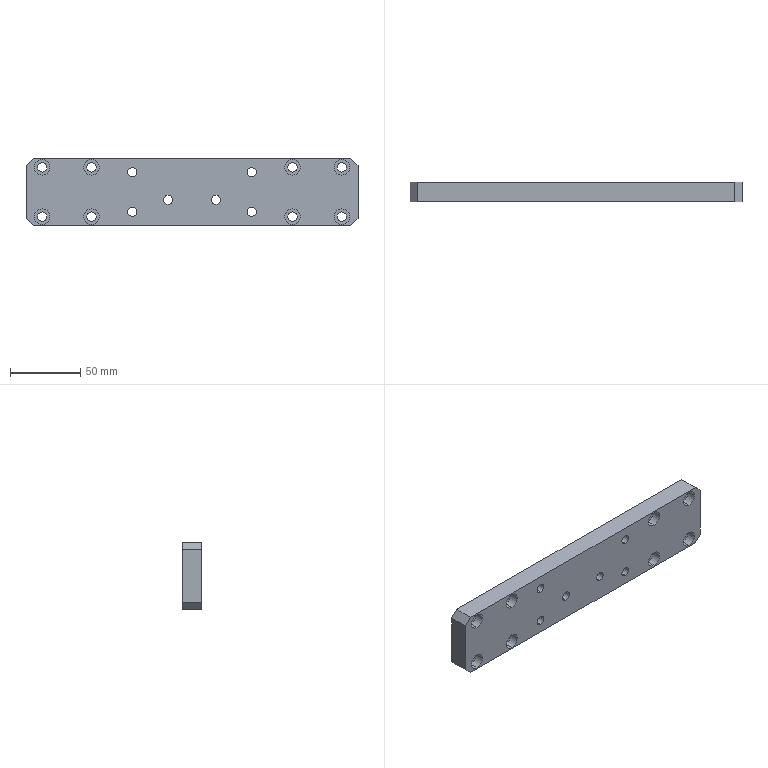Part | SolidWorks | features HoleWzd 3, Chamfer 1, Extrusion 1 | 1 solid | 74 faces | box 236 x 14 x 48 mm | volume 146515 mm3 | cylinder 52 | plane 22 | commonest cylinder face diameters 6.6 x28 11 x24